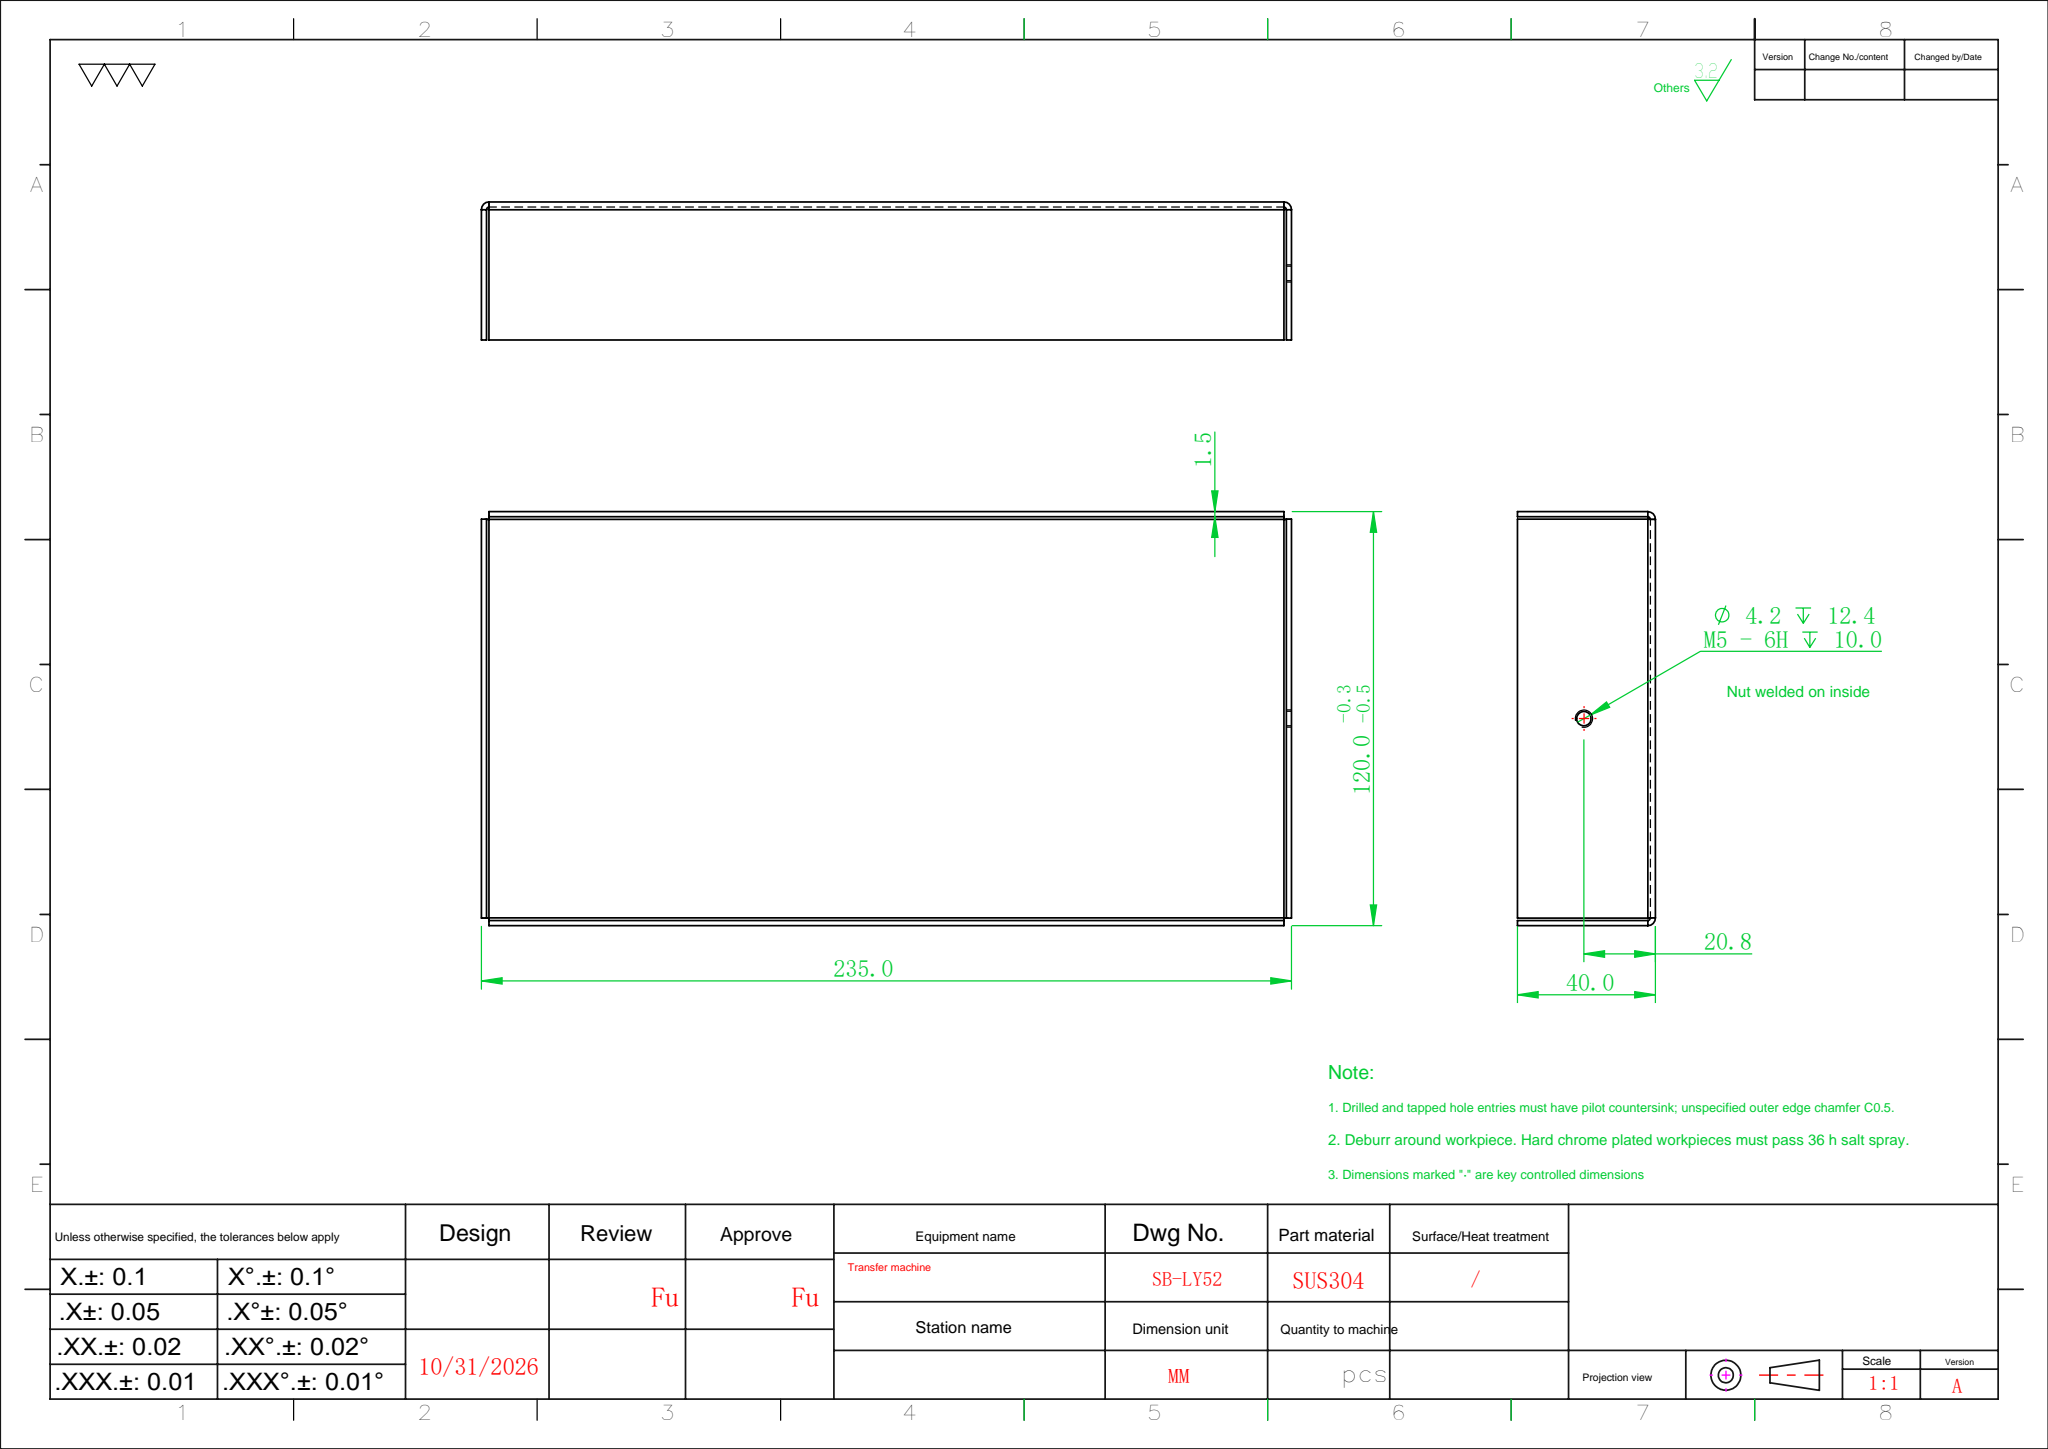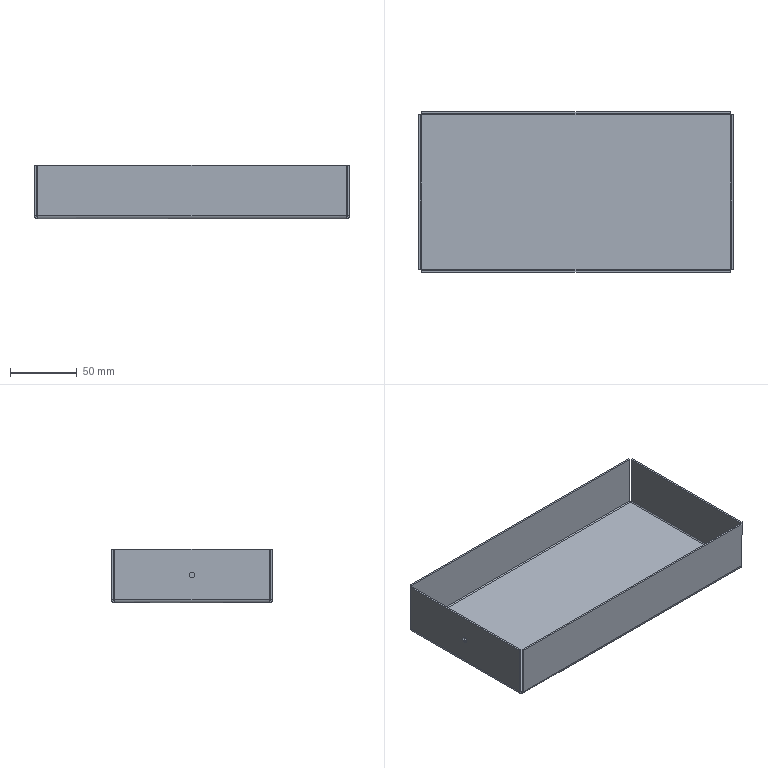Part | SolidWorks | features EdgeFlange 1, FlatPattern 1, HoleWzd 1, SMBaseFlange 1, SheetMetal 1 | 1 solid | 40 faces | box 235 x 120 x 40 mm | volume 81570 mm3 | plane 22 | cylinder 10 | spline 8 | commonest cylinder face diameters 1.473 x4 4.473 x4 4.2 x2